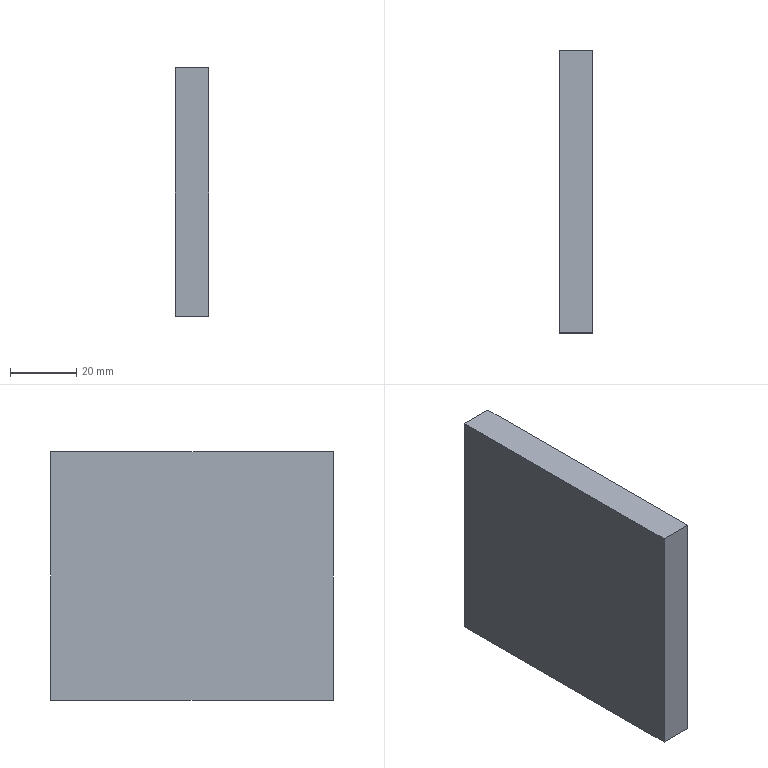Part | NX | features solid 2 | 1 solid | 6 faces | box 10 x 85 x 75 mm | volume 63750 mm3 | plane 6
STEP:
#1=CARTESIAN_POINT('',(940.,422.5,-80.));
#2=VERTEX_POINT('',#1);
#3=CARTESIAN_POINT('',(940.,422.5,-155.));
#4=VERTEX_POINT('',#3);
#5=CARTESIAN_POINT('',(940.,422.5,-80.));
#6=CARTESIAN_POINT('',(940.,422.5,-105.));
#7=CARTESIAN_POINT('',(940.,422.5,-130.));
#8=CARTESIAN_POINT('',(940.,422.5,-155.));
#9=B_SPLINE_CURVE_WITH_KNOTS('',3,(#5,#6,#7,#8),.UNSPECIFIED.,.F.,.F.,(4,4),(0.,1.),.UNSPECIFIED.);
#10=EDGE_CURVE('',#2,#4,#9,.T.);
#11=ORIENTED_EDGE('',*,*,#10,.T.);
#12=CARTESIAN_POINT('',(930.,422.5,-155.));
#13=VERTEX_POINT('',#12);
#14=CARTESIAN_POINT('',(940.,422.5,-155.));
#15=CARTESIAN_POINT('',(936.667,422.5,-155.));
#16=CARTESIAN_POINT('',(933.333,422.5,-155.));
#17=CARTESIAN_POINT('',(930.,422.5,-155.));
#18=B_SPLINE_CURVE_WITH_KNOTS('',3,(#14,#15,#16,#17),.UNSPECIFIED.,.F.,.F.,(4,4),(0.,1.),.UNSPECIFIED.);
#19=EDGE_CURVE('',#13,#4,#18,.F.);
#20=ORIENTED_EDGE('',*,*,#19,.F.);
#21=CARTESIAN_POINT('',(930.,422.5,-80.));
#22=VERTEX_POINT('',#21);
#23=CARTESIAN_POINT('',(930.,422.5,-155.));
#24=CARTESIAN_POINT('',(930.,422.5,-130.));
#25=CARTESIAN_POINT('',(930.,422.5,-105.));
#26=CARTESIAN_POINT('',(930.,422.5,-80.));
#27=B_SPLINE_CURVE_WITH_KNOTS('',3,(#23,#24,#25,#26),.UNSPECIFIED.,.F.,.F.,(4,4),(0.,1.),.UNSPECIFIED.);
#28=EDGE_CURVE('',#22,#13,#27,.F.);
#29=ORIENTED_EDGE('',*,*,#28,.F.);
#30=CARTESIAN_POINT('',(930.,422.5,-80.));
#31=CARTESIAN_POINT('',(933.333,422.5,-80.));
#32=CARTESIAN_POINT('',(936.667,422.5,-80.));
#33=CARTESIAN_POINT('',(940.,422.5,-80.));
#34=B_SPLINE_CURVE_WITH_KNOTS('',3,(#30,#31,#32,#33),.UNSPECIFIED.,.F.,.F.,(4,4),(0.,1.),.UNSPECIFIED.);
#35=EDGE_CURVE('',#22,#2,#34,.T.);
#36=ORIENTED_EDGE('',*,*,#35,.T.);
#37=EDGE_LOOP('',(#11,#20,#29,#36));
#38=FACE_BOUND('',#37,.T.);
#39=CARTESIAN_POINT('',(930.,422.5,-117.5));
#40=DIRECTION('',(0.000000011,1.,-0.00000017));
#41=DIRECTION('',(0.000000341,-0.00000017,-1.));
#42=AXIS2_PLACEMENT_3D('',#39,#40,#41);
#43=PLANE('',#42);
#44=ADVANCED_FACE('',(#38),#43,.T.);
#45=CARTESIAN_POINT('',(940.,337.5,-155.));
#46=VERTEX_POINT('',#45);
#47=CARTESIAN_POINT('',(940.,422.5,-155.));
#48=CARTESIAN_POINT('',(940.,394.167,-155.));
#49=CARTESIAN_POINT('',(940.,365.833,-155.));
#50=CARTESIAN_POINT('',(940.,337.5,-155.));
#51=B_SPLINE_CURVE_WITH_KNOTS('',3,(#47,#48,#49,#50),.UNSPECIFIED.,.F.,.F.,(4,4),(0.,1.),.UNSPECIFIED.);
#52=EDGE_CURVE('',#4,#46,#51,.T.);
#53=ORIENTED_EDGE('',*,*,#52,.T.);
#54=CARTESIAN_POINT('',(930.,337.5,-155.));
#55=VERTEX_POINT('',#54);
#56=CARTESIAN_POINT('',(940.,337.5,-155.));
#57=CARTESIAN_POINT('',(936.667,337.5,-155.));
#58=CARTESIAN_POINT('',(933.333,337.5,-155.));
#59=CARTESIAN_POINT('',(930.,337.5,-155.));
#60=B_SPLINE_CURVE_WITH_KNOTS('',3,(#56,#57,#58,#59),.UNSPECIFIED.,.F.,.F.,(4,4),(0.,1.),.UNSPECIFIED.);
#61=EDGE_CURVE('',#55,#46,#60,.F.);
#62=ORIENTED_EDGE('',*,*,#61,.F.);
#63=CARTESIAN_POINT('',(930.,337.5,-155.));
#64=CARTESIAN_POINT('',(930.,365.833,-155.));
#65=CARTESIAN_POINT('',(930.,394.167,-155.));
#66=CARTESIAN_POINT('',(930.,422.5,-155.));
#67=B_SPLINE_CURVE_WITH_KNOTS('',3,(#63,#64,#65,#66),.UNSPECIFIED.,.F.,.F.,(4,4),(0.,1.),.UNSPECIFIED.);
#68=EDGE_CURVE('',#13,#55,#67,.F.);
#69=ORIENTED_EDGE('',*,*,#68,.F.);
#70=ORIENTED_EDGE('',*,*,#19,.T.);
#71=EDGE_LOOP('',(#53,#62,#69,#70));
#72=FACE_BOUND('',#71,.T.);
#73=CARTESIAN_POINT('',(930.,380.,-155.));
#74=DIRECTION('',(0.000000341,-0.00000017,-1.));
#75=DIRECTION('',(-1.,0.000000011,-0.000000341));
#76=AXIS2_PLACEMENT_3D('',#73,#74,#75);
#77=PLANE('',#76);
#78=ADVANCED_FACE('',(#72),#77,.T.);
#79=CARTESIAN_POINT('',(940.,337.5,-80.));
#80=VERTEX_POINT('',#79);
#81=CARTESIAN_POINT('',(940.,337.5,-155.));
#82=CARTESIAN_POINT('',(940.,337.5,-130.));
#83=CARTESIAN_POINT('',(940.,337.5,-105.));
#84=CARTESIAN_POINT('',(940.,337.5,-80.));
#85=B_SPLINE_CURVE_WITH_KNOTS('',3,(#81,#82,#83,#84),.UNSPECIFIED.,.F.,.F.,(4,4),(0.,1.),.UNSPECIFIED.);
#86=EDGE_CURVE('',#46,#80,#85,.T.);
#87=ORIENTED_EDGE('',*,*,#86,.T.);
#88=CARTESIAN_POINT('',(930.,337.5,-80.));
#89=VERTEX_POINT('',#88);
#90=CARTESIAN_POINT('',(940.,337.5,-80.));
#91=CARTESIAN_POINT('',(936.667,337.5,-80.));
#92=CARTESIAN_POINT('',(933.333,337.5,-80.));
#93=CARTESIAN_POINT('',(930.,337.5,-80.));
#94=B_SPLINE_CURVE_WITH_KNOTS('',3,(#90,#91,#92,#93),.UNSPECIFIED.,.F.,.F.,(4,4),(0.,1.),.UNSPECIFIED.);
#95=EDGE_CURVE('',#89,#80,#94,.F.);
#96=ORIENTED_EDGE('',*,*,#95,.F.);
#97=CARTESIAN_POINT('',(930.,337.5,-80.));
#98=CARTESIAN_POINT('',(930.,337.5,-105.));
#99=CARTESIAN_POINT('',(930.,337.5,-130.));
#100=CARTESIAN_POINT('',(930.,337.5,-155.));
#101=B_SPLINE_CURVE_WITH_KNOTS('',3,(#97,#98,#99,#100),.UNSPECIFIED.,.F.,.F.,(4,4),(0.,1.),.UNSPECIFIED.);
#102=EDGE_CURVE('',#55,#89,#101,.F.);
#103=ORIENTED_EDGE('',*,*,#102,.F.);
#104=ORIENTED_EDGE('',*,*,#61,.T.);
#105=EDGE_LOOP('',(#87,#96,#103,#104));
#106=FACE_BOUND('',#105,.T.);
#107=CARTESIAN_POINT('',(930.,337.5,-117.5));
#108=DIRECTION('',(-0.000000011,-1.,0.00000017));
#109=DIRECTION('',(-0.000000341,0.00000017,1.));
#110=AXIS2_PLACEMENT_3D('',#107,#108,#109);
#111=PLANE('',#110);
#112=ADVANCED_FACE('',(#106),#111,.T.);
#113=CARTESIAN_POINT('',(940.,337.5,-80.));
#114=CARTESIAN_POINT('',(940.,365.833,-80.));
#115=CARTESIAN_POINT('',(940.,394.167,-80.));
#116=CARTESIAN_POINT('',(940.,422.5,-80.));
#117=B_SPLINE_CURVE_WITH_KNOTS('',3,(#113,#114,#115,#116),.UNSPECIFIED.,.F.,.F.,(4,4),(0.,1.),.UNSPECIFIED.);
#118=EDGE_CURVE('',#80,#2,#117,.T.);
#119=ORIENTED_EDGE('',*,*,#118,.T.);
#120=ORIENTED_EDGE('',*,*,#35,.F.);
#121=CARTESIAN_POINT('',(930.,422.5,-80.));
#122=CARTESIAN_POINT('',(930.,394.167,-80.));
#123=CARTESIAN_POINT('',(930.,365.833,-80.));
#124=CARTESIAN_POINT('',(930.,337.5,-80.));
#125=B_SPLINE_CURVE_WITH_KNOTS('',3,(#121,#122,#123,#124),.UNSPECIFIED.,.F.,.F.,(4,4),(0.,1.),.UNSPECIFIED.);
#126=EDGE_CURVE('',#89,#22,#125,.F.);
#127=ORIENTED_EDGE('',*,*,#126,.F.);
#128=ORIENTED_EDGE('',*,*,#95,.T.);
#129=EDGE_LOOP('',(#119,#120,#127,#128));
#130=FACE_BOUND('',#129,.T.);
#131=CARTESIAN_POINT('',(930.,380.,-80.));
#132=DIRECTION('',(-0.000000341,0.00000017,1.));
#133=DIRECTION('',(1.,-0.000000011,0.000000341));
#134=AXIS2_PLACEMENT_3D('',#131,#132,#133);
#135=PLANE('',#134);
#136=ADVANCED_FACE('',(#130),#135,.T.);
#137=ORIENTED_EDGE('',*,*,#28,.T.);
#138=ORIENTED_EDGE('',*,*,#68,.T.);
#139=ORIENTED_EDGE('',*,*,#102,.T.);
#140=ORIENTED_EDGE('',*,*,#126,.T.);
#141=EDGE_LOOP('',(#137,#138,#139,#140));
#142=FACE_BOUND('',#141,.T.);
#143=CARTESIAN_POINT('',(930.,380.,-117.5));
#144=DIRECTION('',(1.,-0.000000011,0.000000341));
#145=DIRECTION('',(-0.000000011,-1.,0.00000017));
#146=AXIS2_PLACEMENT_3D('',#143,#144,#145);
#147=PLANE('',#146);
#148=ADVANCED_FACE('',(#142),#147,.F.);
#149=ORIENTED_EDGE('',*,*,#10,.F.);
#150=ORIENTED_EDGE('',*,*,#118,.F.);
#151=ORIENTED_EDGE('',*,*,#86,.F.);
#152=ORIENTED_EDGE('',*,*,#52,.F.);
#153=EDGE_LOOP('',(#149,#150,#151,#152));
#154=FACE_BOUND('',#153,.T.);
#155=CARTESIAN_POINT('',(940.,380.,-117.5));
#156=DIRECTION('',(1.,-0.000000011,0.000000341));
#157=DIRECTION('',(-0.000000011,-1.,0.00000017));
#158=AXIS2_PLACEMENT_3D('',#155,#156,#157);
#159=PLANE('',#158);
#160=ADVANCED_FACE('',(#154),#159,.T.);
#161=CLOSED_SHELL('',(#44,#78,#112,#136,#148,#160));
#162=MANIFOLD_SOLID_BREP('',#161);
#163=(LENGTH_UNIT()NAMED_UNIT(*)SI_UNIT(.MILLI.,.METRE.));
#164=UNCERTAINTY_MEASURE_WITH_UNIT(LENGTH_MEASURE(0.0508),#163,'','');
#165=(NAMED_UNIT(*)PLANE_ANGLE_UNIT()SI_UNIT($,.RADIAN.));
#166=(NAMED_UNIT(*)SI_UNIT($,.STERADIAN.)SOLID_ANGLE_UNIT());
#167=(GEOMETRIC_REPRESENTATION_CONTEXT(3)GLOBAL_UNCERTAINTY_ASSIGNED_CONTEXT((#164))GLOBAL_UNIT_ASSIGNED_CONTEXT((#163,#165,#166))REPRESENTATION_CONTEXT('',''));
#168=ADVANCED_BREP_SHAPE_REPRESENTATION('',(#162),#167);